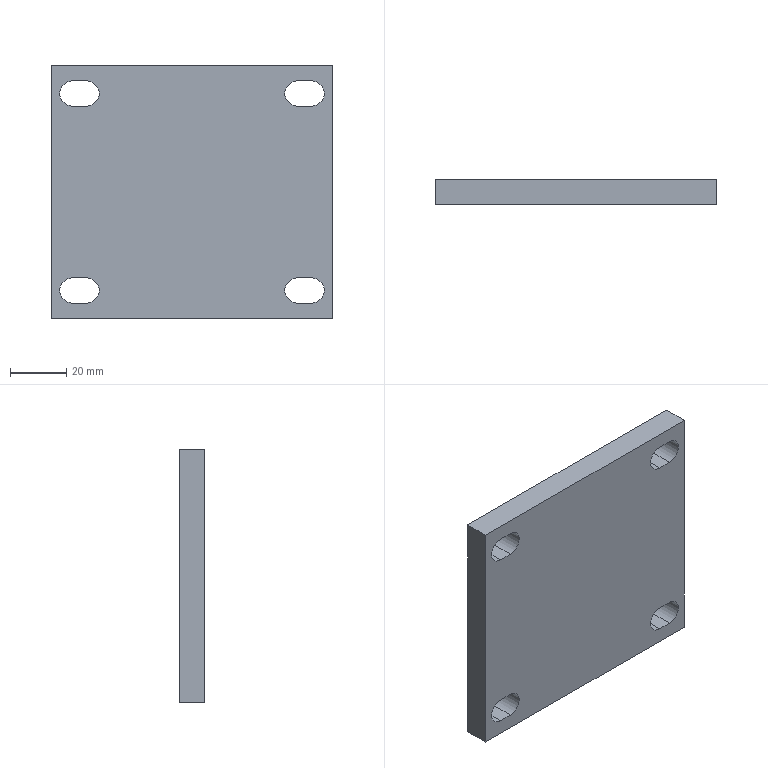Part | STEP file | X77-02211 | 1 solid | 22 faces | box 100 x 9 x 90 mm | volume 77090 mm3 | plane 14 | cylinder 8 | commonest cylinder face diameters 9 x8
STEP:
#1=CARTESIAN_POINT('',(50.,10.,45.));
#2=VERTEX_POINT('',#1);
#3=CARTESIAN_POINT('',(50.,1.,45.));
#4=VERTEX_POINT('',#3);
#5=CARTESIAN_POINT('',(50.,10.,45.));
#6=DIRECTION('',(0.,-1.,0.));
#7=VECTOR('',#6,1000.);
#8=LINE('',#5,#7);
#9=EDGE_CURVE('',#2,#4,#8,.T.);
#10=ORIENTED_EDGE('',*,*,#9,.T.);
#11=CARTESIAN_POINT('',(50.,1.,-45.));
#12=VERTEX_POINT('',#11);
#13=CARTESIAN_POINT('',(50.,1.,45.));
#14=DIRECTION('',(0.,0.,1.));
#15=VECTOR('',#14,1000.);
#16=LINE('',#13,#15);
#17=EDGE_CURVE('',#12,#4,#16,.T.);
#18=ORIENTED_EDGE('',*,*,#17,.F.);
#19=CARTESIAN_POINT('',(50.,10.,-45.));
#20=VERTEX_POINT('',#19);
#21=CARTESIAN_POINT('',(50.,10.,-45.));
#22=DIRECTION('',(0.,-1.,0.));
#23=VECTOR('',#22,1000.);
#24=LINE('',#21,#23);
#25=EDGE_CURVE('',#20,#12,#24,.T.);
#26=ORIENTED_EDGE('',*,*,#25,.F.);
#27=CARTESIAN_POINT('',(50.,10.,45.));
#28=DIRECTION('',(0.,0.,-1.));
#29=VECTOR('',#28,1000.);
#30=LINE('',#27,#29);
#31=EDGE_CURVE('',#2,#20,#30,.T.);
#32=ORIENTED_EDGE('',*,*,#31,.F.);
#33=EDGE_LOOP('',(#10,#18,#26,#32));
#34=FACE_OUTER_BOUND('',#33,.T.);
#35=CARTESIAN_POINT('',(50.,10.,45.));
#36=DIRECTION('',(-1.,0.,0.));
#37=DIRECTION('',(0.,0.,1.));
#38=AXIS2_PLACEMENT_3D('',#35,#36,#37);
#39=PLANE('',#38);
#40=ADVANCED_FACE('',(#34),#39,.F.);
#41=ORIENTED_EDGE('',*,*,#25,.T.);
#42=CARTESIAN_POINT('',(-50.,1.,-45.));
#43=VERTEX_POINT('',#42);
#44=CARTESIAN_POINT('',(-50.,1.,-45.));
#45=DIRECTION('',(1.,0.,0.));
#46=VECTOR('',#45,1000.);
#47=LINE('',#44,#46);
#48=EDGE_CURVE('',#43,#12,#47,.T.);
#49=ORIENTED_EDGE('',*,*,#48,.F.);
#50=CARTESIAN_POINT('',(-50.,10.,-45.));
#51=VERTEX_POINT('',#50);
#52=CARTESIAN_POINT('',(-50.,10.,-45.));
#53=DIRECTION('',(0.,-1.,0.));
#54=VECTOR('',#53,1000.);
#55=LINE('',#52,#54);
#56=EDGE_CURVE('',#51,#43,#55,.T.);
#57=ORIENTED_EDGE('',*,*,#56,.F.);
#58=CARTESIAN_POINT('',(-50.,10.,-45.));
#59=DIRECTION('',(-1.,0.,0.));
#60=VECTOR('',#59,1000.);
#61=LINE('',#58,#60);
#62=EDGE_CURVE('',#20,#51,#61,.T.);
#63=ORIENTED_EDGE('',*,*,#62,.F.);
#64=EDGE_LOOP('',(#41,#49,#57,#63));
#65=FACE_OUTER_BOUND('',#64,.T.);
#66=CARTESIAN_POINT('',(-50.,10.,-45.));
#67=DIRECTION('',(0.,0.,1.));
#68=DIRECTION('',(1.,0.,0.));
#69=AXIS2_PLACEMENT_3D('',#66,#67,#68);
#70=PLANE('',#69);
#71=ADVANCED_FACE('',(#65),#70,.F.);
#72=ORIENTED_EDGE('',*,*,#56,.T.);
#73=CARTESIAN_POINT('',(-50.,1.,45.));
#74=VERTEX_POINT('',#73);
#75=CARTESIAN_POINT('',(-50.,1.,45.));
#76=DIRECTION('',(0.,0.,1.));
#77=VECTOR('',#76,1000.);
#78=LINE('',#75,#77);
#79=EDGE_CURVE('',#43,#74,#78,.T.);
#80=ORIENTED_EDGE('',*,*,#79,.T.);
#81=CARTESIAN_POINT('',(-50.,10.,45.));
#82=VERTEX_POINT('',#81);
#83=CARTESIAN_POINT('',(-50.,10.,45.));
#84=DIRECTION('',(0.,-1.,0.));
#85=VECTOR('',#84,1000.);
#86=LINE('',#83,#85);
#87=EDGE_CURVE('',#82,#74,#86,.T.);
#88=ORIENTED_EDGE('',*,*,#87,.F.);
#89=CARTESIAN_POINT('',(-50.,10.,45.));
#90=DIRECTION('',(0.,0.,1.));
#91=VECTOR('',#90,1000.);
#92=LINE('',#89,#91);
#93=EDGE_CURVE('',#51,#82,#92,.T.);
#94=ORIENTED_EDGE('',*,*,#93,.F.);
#95=EDGE_LOOP('',(#72,#80,#88,#94));
#96=FACE_OUTER_BOUND('',#95,.T.);
#97=CARTESIAN_POINT('',(-50.,10.,45.));
#98=DIRECTION('',(1.,0.,0.));
#99=DIRECTION('',(0.,0.,-1.));
#100=AXIS2_PLACEMENT_3D('',#97,#98,#99);
#101=PLANE('',#100);
#102=ADVANCED_FACE('',(#96),#101,.F.);
#103=ORIENTED_EDGE('',*,*,#87,.T.);
#104=CARTESIAN_POINT('',(-50.,1.,45.));
#105=DIRECTION('',(1.,0.,0.));
#106=VECTOR('',#105,1000.);
#107=LINE('',#104,#106);
#108=EDGE_CURVE('',#74,#4,#107,.T.);
#109=ORIENTED_EDGE('',*,*,#108,.T.);
#110=ORIENTED_EDGE('',*,*,#9,.F.);
#111=CARTESIAN_POINT('',(-50.,10.,45.));
#112=DIRECTION('',(1.,0.,0.));
#113=VECTOR('',#112,1000.);
#114=LINE('',#111,#113);
#115=EDGE_CURVE('',#82,#2,#114,.T.);
#116=ORIENTED_EDGE('',*,*,#115,.F.);
#117=EDGE_LOOP('',(#103,#109,#110,#116));
#118=FACE_OUTER_BOUND('',#117,.T.);
#119=CARTESIAN_POINT('',(-50.,10.,45.));
#120=DIRECTION('',(0.,0.,-1.));
#121=DIRECTION('',(-1.,0.,0.));
#122=AXIS2_PLACEMENT_3D('',#119,#120,#121);
#123=PLANE('',#122);
#124=ADVANCED_FACE('',(#118),#123,.F.);
#125=CARTESIAN_POINT('',(42.5,10.,-39.5));
#126=VERTEX_POINT('',#125);
#127=CARTESIAN_POINT('',(37.5,10.,-39.5));
#128=VERTEX_POINT('',#127);
#129=CARTESIAN_POINT('',(42.5,10.,-39.5));
#130=DIRECTION('',(-1.,0.,0.));
#131=VECTOR('',#130,1000.);
#132=LINE('',#129,#131);
#133=EDGE_CURVE('',#126,#128,#132,.T.);
#134=ORIENTED_EDGE('',*,*,#133,.F.);
#135=CARTESIAN_POINT('',(42.5,10.,-30.5));
#136=VERTEX_POINT('',#135);
#137=CARTESIAN_POINT('',(42.5,10.,-35.));
#138=DIRECTION('',(0.,1.,0.));
#139=DIRECTION('',(0.,0.,1.));
#140=AXIS2_PLACEMENT_3D('',#137,#138,#139);
#141=CIRCLE('',#140,4.5);
#142=EDGE_CURVE('',#136,#126,#141,.T.);
#143=ORIENTED_EDGE('',*,*,#142,.F.);
#144=CARTESIAN_POINT('',(37.5,10.,-30.5));
#145=VERTEX_POINT('',#144);
#146=CARTESIAN_POINT('',(42.5,10.,-30.5));
#147=DIRECTION('',(1.,0.,0.));
#148=VECTOR('',#147,1000.);
#149=LINE('',#146,#148);
#150=EDGE_CURVE('',#145,#136,#149,.T.);
#151=ORIENTED_EDGE('',*,*,#150,.F.);
#152=CARTESIAN_POINT('',(37.5,10.,-35.));
#153=DIRECTION('',(0.,1.,0.));
#154=DIRECTION('',(0.,0.,1.));
#155=AXIS2_PLACEMENT_3D('',#152,#153,#154);
#156=CIRCLE('',#155,4.5);
#157=EDGE_CURVE('',#128,#145,#156,.T.);
#158=ORIENTED_EDGE('',*,*,#157,.F.);
#159=EDGE_LOOP('',(#134,#143,#151,#158));
#160=FACE_BOUND('',#159,.T.);
#161=CARTESIAN_POINT('',(-37.5,10.,-39.5));
#162=VERTEX_POINT('',#161);
#163=CARTESIAN_POINT('',(-42.5,10.,-39.5));
#164=VERTEX_POINT('',#163);
#165=CARTESIAN_POINT('',(-37.5,10.,-39.5));
#166=DIRECTION('',(-1.,0.,0.));
#167=VECTOR('',#166,1000.);
#168=LINE('',#165,#167);
#169=EDGE_CURVE('',#162,#164,#168,.T.);
#170=ORIENTED_EDGE('',*,*,#169,.F.);
#171=CARTESIAN_POINT('',(-37.5,10.,-30.5));
#172=VERTEX_POINT('',#171);
#173=CARTESIAN_POINT('',(-37.5,10.,-35.));
#174=DIRECTION('',(0.,1.,0.));
#175=DIRECTION('',(0.,0.,1.));
#176=AXIS2_PLACEMENT_3D('',#173,#174,#175);
#177=CIRCLE('',#176,4.5);
#178=EDGE_CURVE('',#172,#162,#177,.T.);
#179=ORIENTED_EDGE('',*,*,#178,.F.);
#180=CARTESIAN_POINT('',(-42.5,10.,-30.5));
#181=VERTEX_POINT('',#180);
#182=CARTESIAN_POINT('',(-37.5,10.,-30.5));
#183=DIRECTION('',(1.,0.,0.));
#184=VECTOR('',#183,1000.);
#185=LINE('',#182,#184);
#186=EDGE_CURVE('',#181,#172,#185,.T.);
#187=ORIENTED_EDGE('',*,*,#186,.F.);
#188=CARTESIAN_POINT('',(-42.5,10.,-35.));
#189=DIRECTION('',(0.,1.,0.));
#190=DIRECTION('',(0.,0.,1.));
#191=AXIS2_PLACEMENT_3D('',#188,#189,#190);
#192=CIRCLE('',#191,4.5);
#193=EDGE_CURVE('',#164,#181,#192,.T.);
#194=ORIENTED_EDGE('',*,*,#193,.F.);
#195=EDGE_LOOP('',(#170,#179,#187,#194));
#196=FACE_BOUND('',#195,.T.);
#197=ORIENTED_EDGE('',*,*,#31,.T.);
#198=ORIENTED_EDGE('',*,*,#62,.T.);
#199=ORIENTED_EDGE('',*,*,#93,.T.);
#200=ORIENTED_EDGE('',*,*,#115,.T.);
#201=EDGE_LOOP('',(#197,#198,#199,#200));
#202=FACE_OUTER_BOUND('',#201,.T.);
#203=CARTESIAN_POINT('',(-37.5,10.,39.5));
#204=VERTEX_POINT('',#203);
#205=CARTESIAN_POINT('',(-37.5,10.,30.5));
#206=VERTEX_POINT('',#205);
#207=CARTESIAN_POINT('',(-37.5,10.,35.));
#208=DIRECTION('',(0.,1.,0.));
#209=DIRECTION('',(0.,0.,1.));
#210=AXIS2_PLACEMENT_3D('',#207,#208,#209);
#211=CIRCLE('',#210,4.5);
#212=EDGE_CURVE('',#204,#206,#211,.T.);
#213=ORIENTED_EDGE('',*,*,#212,.F.);
#214=CARTESIAN_POINT('',(-42.5,10.,39.5));
#215=VERTEX_POINT('',#214);
#216=CARTESIAN_POINT('',(-37.5,10.,39.5));
#217=DIRECTION('',(1.,0.,0.));
#218=VECTOR('',#217,1000.);
#219=LINE('',#216,#218);
#220=EDGE_CURVE('',#215,#204,#219,.T.);
#221=ORIENTED_EDGE('',*,*,#220,.F.);
#222=CARTESIAN_POINT('',(-42.5,10.,30.5));
#223=VERTEX_POINT('',#222);
#224=CARTESIAN_POINT('',(-42.5,10.,35.));
#225=DIRECTION('',(0.,1.,0.));
#226=DIRECTION('',(0.,0.,1.));
#227=AXIS2_PLACEMENT_3D('',#224,#225,#226);
#228=CIRCLE('',#227,4.5);
#229=EDGE_CURVE('',#223,#215,#228,.T.);
#230=ORIENTED_EDGE('',*,*,#229,.F.);
#231=CARTESIAN_POINT('',(-37.5,10.,30.5));
#232=DIRECTION('',(-1.,0.,0.));
#233=VECTOR('',#232,1000.);
#234=LINE('',#231,#233);
#235=EDGE_CURVE('',#206,#223,#234,.T.);
#236=ORIENTED_EDGE('',*,*,#235,.F.);
#237=EDGE_LOOP('',(#213,#221,#230,#236));
#238=FACE_BOUND('',#237,.T.);
#239=CARTESIAN_POINT('',(42.5,10.,39.5));
#240=VERTEX_POINT('',#239);
#241=CARTESIAN_POINT('',(42.5,10.,30.5));
#242=VERTEX_POINT('',#241);
#243=CARTESIAN_POINT('',(42.5,10.,35.));
#244=DIRECTION('',(0.,1.,0.));
#245=DIRECTION('',(0.,0.,1.));
#246=AXIS2_PLACEMENT_3D('',#243,#244,#245);
#247=CIRCLE('',#246,4.5);
#248=EDGE_CURVE('',#240,#242,#247,.T.);
#249=ORIENTED_EDGE('',*,*,#248,.F.);
#250=CARTESIAN_POINT('',(37.5,10.,39.5));
#251=VERTEX_POINT('',#250);
#252=CARTESIAN_POINT('',(42.5,10.,39.5));
#253=DIRECTION('',(1.,0.,0.));
#254=VECTOR('',#253,1000.);
#255=LINE('',#252,#254);
#256=EDGE_CURVE('',#251,#240,#255,.T.);
#257=ORIENTED_EDGE('',*,*,#256,.F.);
#258=CARTESIAN_POINT('',(37.5,10.,30.5));
#259=VERTEX_POINT('',#258);
#260=CARTESIAN_POINT('',(37.5,10.,35.));
#261=DIRECTION('',(0.,1.,0.));
#262=DIRECTION('',(0.,0.,1.));
#263=AXIS2_PLACEMENT_3D('',#260,#261,#262);
#264=CIRCLE('',#263,4.5);
#265=EDGE_CURVE('',#259,#251,#264,.T.);
#266=ORIENTED_EDGE('',*,*,#265,.F.);
#267=CARTESIAN_POINT('',(42.5,10.,30.5));
#268=DIRECTION('',(-1.,0.,0.));
#269=VECTOR('',#268,1000.);
#270=LINE('',#267,#269);
#271=EDGE_CURVE('',#242,#259,#270,.T.);
#272=ORIENTED_EDGE('',*,*,#271,.F.);
#273=EDGE_LOOP('',(#249,#257,#266,#272));
#274=FACE_BOUND('',#273,.T.);
#275=CARTESIAN_POINT('',(50.,10.,-45.));
#276=DIRECTION('',(0.,-1.,0.));
#277=DIRECTION('',(0.,0.,-1.));
#278=AXIS2_PLACEMENT_3D('',#275,#276,#277);
#279=PLANE('',#278);
#280=ADVANCED_FACE('',(#160,#196,#202,#238,#274),#279,.F.);
#281=CARTESIAN_POINT('',(-37.5,1.,-39.5));
#282=VERTEX_POINT('',#281);
#283=CARTESIAN_POINT('',(-37.5,0.,-39.5));
#284=DIRECTION('',(0.,1.,0.));
#285=VECTOR('',#284,1000.);
#286=LINE('',#283,#285);
#287=EDGE_CURVE('',#282,#162,#286,.T.);
#288=ORIENTED_EDGE('',*,*,#287,.F.);
#289=CARTESIAN_POINT('',(-37.5,1.,-30.5));
#290=VERTEX_POINT('',#289);
#291=CARTESIAN_POINT('',(-37.5,1.,-35.));
#292=DIRECTION('',(0.,-1.,0.));
#293=DIRECTION('',(0.,0.,1.));
#294=AXIS2_PLACEMENT_3D('',#291,#292,#293);
#295=CIRCLE('',#294,4.5);
#296=EDGE_CURVE('',#282,#290,#295,.T.);
#297=ORIENTED_EDGE('',*,*,#296,.T.);
#298=CARTESIAN_POINT('',(-37.5,0.,-30.5));
#299=DIRECTION('',(0.,1.,0.));
#300=VECTOR('',#299,1000.);
#301=LINE('',#298,#300);
#302=EDGE_CURVE('',#290,#172,#301,.T.);
#303=ORIENTED_EDGE('',*,*,#302,.T.);
#304=ORIENTED_EDGE('',*,*,#178,.T.);
#305=EDGE_LOOP('',(#288,#297,#303,#304));
#306=FACE_OUTER_BOUND('',#305,.T.);
#307=CARTESIAN_POINT('',(-37.5,0.,-35.));
#308=DIRECTION('',(0.,1.,0.));
#309=DIRECTION('',(0.,0.,1.));
#310=AXIS2_PLACEMENT_3D('',#307,#308,#309);
#311=CYLINDRICAL_SURFACE('',#310,4.5);
#312=ADVANCED_FACE('',(#306),#311,.F.);
#313=ORIENTED_EDGE('',*,*,#302,.F.);
#314=CARTESIAN_POINT('',(-42.5,1.,-30.5));
#315=VERTEX_POINT('',#314);
#316=CARTESIAN_POINT('',(-37.5,1.,-30.5));
#317=DIRECTION('',(-1.,0.,0.));
#318=VECTOR('',#317,1000.);
#319=LINE('',#316,#318);
#320=EDGE_CURVE('',#290,#315,#319,.T.);
#321=ORIENTED_EDGE('',*,*,#320,.T.);
#322=CARTESIAN_POINT('',(-42.5,0.,-30.5));
#323=DIRECTION('',(0.,1.,0.));
#324=VECTOR('',#323,1000.);
#325=LINE('',#322,#324);
#326=EDGE_CURVE('',#315,#181,#325,.T.);
#327=ORIENTED_EDGE('',*,*,#326,.T.);
#328=ORIENTED_EDGE('',*,*,#186,.T.);
#329=EDGE_LOOP('',(#313,#321,#327,#328));
#330=FACE_OUTER_BOUND('',#329,.T.);
#331=CARTESIAN_POINT('',(-37.5,0.,-30.5));
#332=DIRECTION('',(0.,0.,1.));
#333=DIRECTION('',(1.,0.,0.));
#334=AXIS2_PLACEMENT_3D('',#331,#332,#333);
#335=PLANE('',#334);
#336=ADVANCED_FACE('',(#330),#335,.F.);
#337=ORIENTED_EDGE('',*,*,#326,.F.);
#338=CARTESIAN_POINT('',(-42.5,1.,-39.5));
#339=VERTEX_POINT('',#338);
#340=CARTESIAN_POINT('',(-42.5,1.,-35.));
#341=DIRECTION('',(0.,-1.,0.));
#342=DIRECTION('',(0.,0.,1.));
#343=AXIS2_PLACEMENT_3D('',#340,#341,#342);
#344=CIRCLE('',#343,4.5);
#345=EDGE_CURVE('',#315,#339,#344,.T.);
#346=ORIENTED_EDGE('',*,*,#345,.T.);
#347=CARTESIAN_POINT('',(-42.5,0.,-39.5));
#348=DIRECTION('',(0.,1.,0.));
#349=VECTOR('',#348,1000.);
#350=LINE('',#347,#349);
#351=EDGE_CURVE('',#339,#164,#350,.T.);
#352=ORIENTED_EDGE('',*,*,#351,.T.);
#353=ORIENTED_EDGE('',*,*,#193,.T.);
#354=EDGE_LOOP('',(#337,#346,#352,#353));
#355=FACE_OUTER_BOUND('',#354,.T.);
#356=CARTESIAN_POINT('',(-42.5,0.,-35.));
#357=DIRECTION('',(0.,1.,0.));
#358=DIRECTION('',(0.,0.,1.));
#359=AXIS2_PLACEMENT_3D('',#356,#357,#358);
#360=CYLINDRICAL_SURFACE('',#359,4.5);
#361=ADVANCED_FACE('',(#355),#360,.F.);
#362=ORIENTED_EDGE('',*,*,#351,.F.);
#363=CARTESIAN_POINT('',(-37.5,1.,-39.5));
#364=DIRECTION('',(1.,0.,0.));
#365=VECTOR('',#364,1000.);
#366=LINE('',#363,#365);
#367=EDGE_CURVE('',#339,#282,#366,.T.);
#368=ORIENTED_EDGE('',*,*,#367,.T.);
#369=ORIENTED_EDGE('',*,*,#287,.T.);
#370=ORIENTED_EDGE('',*,*,#169,.T.);
#371=EDGE_LOOP('',(#362,#368,#369,#370));
#372=FACE_OUTER_BOUND('',#371,.T.);
#373=CARTESIAN_POINT('',(-37.5,0.,-39.5));
#374=DIRECTION('',(0.,0.,-1.));
#375=DIRECTION('',(-1.,0.,0.));
#376=AXIS2_PLACEMENT_3D('',#373,#374,#375);
#377=PLANE('',#376);
#378=ADVANCED_FACE('',(#372),#377,.F.);
#379=CARTESIAN_POINT('',(37.5,1.,-39.5));
#380=VERTEX_POINT('',#379);
#381=CARTESIAN_POINT('',(37.5,0.,-39.5));
#382=DIRECTION('',(0.,1.,0.));
#383=VECTOR('',#382,1000.);
#384=LINE('',#381,#383);
#385=EDGE_CURVE('',#380,#128,#384,.T.);
#386=ORIENTED_EDGE('',*,*,#385,.F.);
#387=CARTESIAN_POINT('',(42.5,1.,-39.5));
#388=VERTEX_POINT('',#387);
#389=CARTESIAN_POINT('',(42.5,1.,-39.5));
#390=DIRECTION('',(1.,0.,0.));
#391=VECTOR('',#390,1000.);
#392=LINE('',#389,#391);
#393=EDGE_CURVE('',#380,#388,#392,.T.);
#394=ORIENTED_EDGE('',*,*,#393,.T.);
#395=CARTESIAN_POINT('',(42.5,0.,-39.5));
#396=DIRECTION('',(0.,1.,0.));
#397=VECTOR('',#396,1000.);
#398=LINE('',#395,#397);
#399=EDGE_CURVE('',#388,#126,#398,.T.);
#400=ORIENTED_EDGE('',*,*,#399,.T.);
#401=ORIENTED_EDGE('',*,*,#133,.T.);
#402=EDGE_LOOP('',(#386,#394,#400,#401));
#403=FACE_OUTER_BOUND('',#402,.T.);
#404=CARTESIAN_POINT('',(42.5,0.,-39.5));
#405=DIRECTION('',(0.,0.,-1.));
#406=DIRECTION('',(-1.,0.,0.));
#407=AXIS2_PLACEMENT_3D('',#404,#405,#406);
#408=PLANE('',#407);
#409=ADVANCED_FACE('',(#403),#408,.F.);
#410=CARTESIAN_POINT('',(37.5,1.,-30.5));
#411=VERTEX_POINT('',#410);
#412=CARTESIAN_POINT('',(37.5,0.,-30.5));
#413=DIRECTION('',(0.,1.,0.));
#414=VECTOR('',#413,1000.);
#415=LINE('',#412,#414);
#416=EDGE_CURVE('',#411,#145,#415,.T.);
#417=ORIENTED_EDGE('',*,*,#416,.F.);
#418=CARTESIAN_POINT('',(37.5,1.,-35.));
#419=DIRECTION('',(0.,-1.,0.));
#420=DIRECTION('',(0.,0.,1.));
#421=AXIS2_PLACEMENT_3D('',#418,#419,#420);
#422=CIRCLE('',#421,4.5);
#423=EDGE_CURVE('',#411,#380,#422,.T.);
#424=ORIENTED_EDGE('',*,*,#423,.T.);
#425=ORIENTED_EDGE('',*,*,#385,.T.);
#426=ORIENTED_EDGE('',*,*,#157,.T.);
#427=EDGE_LOOP('',(#417,#424,#425,#426));
#428=FACE_OUTER_BOUND('',#427,.T.);
#429=CARTESIAN_POINT('',(37.5,0.,-35.));
#430=DIRECTION('',(0.,1.,0.));
#431=DIRECTION('',(0.,0.,1.));
#432=AXIS2_PLACEMENT_3D('',#429,#430,#431);
#433=CYLINDRICAL_SURFACE('',#432,4.5);
#434=ADVANCED_FACE('',(#428),#433,.F.);
#435=CARTESIAN_POINT('',(42.5,1.,-30.5));
#436=VERTEX_POINT('',#435);
#437=CARTESIAN_POINT('',(42.5,0.,-30.5));
#438=DIRECTION('',(0.,1.,0.));
#439=VECTOR('',#438,1000.);
#440=LINE('',#437,#439);
#441=EDGE_CURVE('',#436,#136,#440,.T.);
#442=ORIENTED_EDGE('',*,*,#441,.F.);
#443=CARTESIAN_POINT('',(42.5,1.,-30.5));
#444=DIRECTION('',(-1.,0.,0.));
#445=VECTOR('',#444,1000.);
#446=LINE('',#443,#445);
#447=EDGE_CURVE('',#436,#411,#446,.T.);
#448=ORIENTED_EDGE('',*,*,#447,.T.);
#449=ORIENTED_EDGE('',*,*,#416,.T.);
#450=ORIENTED_EDGE('',*,*,#150,.T.);
#451=EDGE_LOOP('',(#442,#448,#449,#450));
#452=FACE_OUTER_BOUND('',#451,.T.);
#453=CARTESIAN_POINT('',(42.5,0.,-30.5));
#454=DIRECTION('',(0.,0.,1.));
#455=DIRECTION('',(1.,0.,0.));
#456=AXIS2_PLACEMENT_3D('',#453,#454,#455);
#457=PLANE('',#456);
#458=ADVANCED_FACE('',(#452),#457,.F.);
#459=ORIENTED_EDGE('',*,*,#399,.F.);
#460=CARTESIAN_POINT('',(42.5,1.,-35.));
#461=DIRECTION('',(0.,-1.,0.));
#462=DIRECTION('',(0.,0.,1.));
#463=AXIS2_PLACEMENT_3D('',#460,#461,#462);
#464=CIRCLE('',#463,4.5);
#465=EDGE_CURVE('',#388,#436,#464,.T.);
#466=ORIENTED_EDGE('',*,*,#465,.T.);
#467=ORIENTED_EDGE('',*,*,#441,.T.);
#468=ORIENTED_EDGE('',*,*,#142,.T.);
#469=EDGE_LOOP('',(#459,#466,#467,#468));
#470=FACE_OUTER_BOUND('',#469,.T.);
#471=CARTESIAN_POINT('',(42.5,0.,-35.));
#472=DIRECTION('',(0.,1.,0.));
#473=DIRECTION('',(0.,0.,1.));
#474=AXIS2_PLACEMENT_3D('',#471,#472,#473);
#475=CYLINDRICAL_SURFACE('',#474,4.5);
#476=ADVANCED_FACE('',(#470),#475,.F.);
#477=CARTESIAN_POINT('',(-42.5,1.,30.5));
#478=VERTEX_POINT('',#477);
#479=CARTESIAN_POINT('',(-42.5,0.,30.5));
#480=DIRECTION('',(0.,1.,0.));
#481=VECTOR('',#480,1000.);
#482=LINE('',#479,#481);
#483=EDGE_CURVE('',#478,#223,#482,.T.);
#484=ORIENTED_EDGE('',*,*,#483,.F.);
#485=CARTESIAN_POINT('',(-37.5,1.,30.5));
#486=VERTEX_POINT('',#485);
#487=CARTESIAN_POINT('',(-37.5,1.,30.5));
#488=DIRECTION('',(1.,0.,0.));
#489=VECTOR('',#488,1000.);
#490=LINE('',#487,#489);
#491=EDGE_CURVE('',#478,#486,#490,.T.);
#492=ORIENTED_EDGE('',*,*,#491,.T.);
#493=CARTESIAN_POINT('',(-37.5,0.,30.5));
#494=DIRECTION('',(0.,1.,0.));
#495=VECTOR('',#494,1000.);
#496=LINE('',#493,#495);
#497=EDGE_CURVE('',#486,#206,#496,.T.);
#498=ORIENTED_EDGE('',*,*,#497,.T.);
#499=ORIENTED_EDGE('',*,*,#235,.T.);
#500=EDGE_LOOP('',(#484,#492,#498,#499));
#501=FACE_OUTER_BOUND('',#500,.T.);
#502=CARTESIAN_POINT('',(-37.5,0.,30.5));
#503=DIRECTION('',(0.,0.,-1.));
#504=DIRECTION('',(-1.,0.,0.));
#505=AXIS2_PLACEMENT_3D('',#502,#503,#504);
#506=PLANE('',#505);
#507=ADVANCED_FACE('',(#501),#506,.F.);
#508=CARTESIAN_POINT('',(-42.5,1.,39.5));
#509=VERTEX_POINT('',#508);
#510=CARTESIAN_POINT('',(-42.5,0.,39.5));
#511=DIRECTION('',(0.,1.,0.));
#512=VECTOR('',#511,1000.);
#513=LINE('',#510,#512);
#514=EDGE_CURVE('',#509,#215,#513,.T.);
#515=ORIENTED_EDGE('',*,*,#514,.F.);
#516=CARTESIAN_POINT('',(-42.5,1.,35.));
#517=DIRECTION('',(0.,-1.,0.));
#518=DIRECTION('',(0.,0.,1.));
#519=AXIS2_PLACEMENT_3D('',#516,#517,#518);
#520=CIRCLE('',#519,4.5);
#521=EDGE_CURVE('',#509,#478,#520,.T.);
#522=ORIENTED_EDGE('',*,*,#521,.T.);
#523=ORIENTED_EDGE('',*,*,#483,.T.);
#524=ORIENTED_EDGE('',*,*,#229,.T.);
#525=EDGE_LOOP('',(#515,#522,#523,#524));
#526=FACE_OUTER_BOUND('',#525,.T.);
#527=CARTESIAN_POINT('',(-42.5,0.,35.));
#528=DIRECTION('',(0.,1.,0.));
#529=DIRECTION('',(0.,0.,1.));
#530=AXIS2_PLACEMENT_3D('',#527,#528,#529);
#531=CYLINDRICAL_SURFACE('',#530,4.5);
#532=ADVANCED_FACE('',(#526),#531,.F.);
#533=CARTESIAN_POINT('',(-37.5,1.,39.5));
#534=VERTEX_POINT('',#533);
#535=CARTESIAN_POINT('',(-37.5,0.,39.5));
#536=DIRECTION('',(0.,1.,0.));
#537=VECTOR('',#536,1000.);
#538=LINE('',#535,#537);
#539=EDGE_CURVE('',#534,#204,#538,.T.);
#540=ORIENTED_EDGE('',*,*,#539,.F.);
#541=CARTESIAN_POINT('',(-37.5,1.,39.5));
#542=DIRECTION('',(-1.,0.,0.));
#543=VECTOR('',#542,1000.);
#544=LINE('',#541,#543);
#545=EDGE_CURVE('',#534,#509,#544,.T.);
#546=ORIENTED_EDGE('',*,*,#545,.T.);
#547=ORIENTED_EDGE('',*,*,#514,.T.);
#548=ORIENTED_EDGE('',*,*,#220,.T.);
#549=EDGE_LOOP('',(#540,#546,#547,#548));
#550=FACE_OUTER_BOUND('',#549,.T.);
#551=CARTESIAN_POINT('',(-37.5,0.,39.5));
#552=DIRECTION('',(0.,0.,1.));
#553=DIRECTION('',(1.,0.,0.));
#554=AXIS2_PLACEMENT_3D('',#551,#552,#553);
#555=PLANE('',#554);
#556=ADVANCED_FACE('',(#550),#555,.F.);
#557=ORIENTED_EDGE('',*,*,#497,.F.);
#558=CARTESIAN_POINT('',(-37.5,1.,35.));
#559=DIRECTION('',(0.,-1.,0.));
#560=DIRECTION('',(0.,0.,1.));
#561=AXIS2_PLACEMENT_3D('',#558,#559,#560);
#562=CIRCLE('',#561,4.5);
#563=EDGE_CURVE('',#486,#534,#562,.T.);
#564=ORIENTED_EDGE('',*,*,#563,.T.);
#565=ORIENTED_EDGE('',*,*,#539,.T.);
#566=ORIENTED_EDGE('',*,*,#212,.T.);
#567=EDGE_LOOP('',(#557,#564,#565,#566));
#568=FACE_OUTER_BOUND('',#567,.T.);
#569=CARTESIAN_POINT('',(-37.5,0.,35.));
#570=DIRECTION('',(0.,1.,0.));
#571=DIRECTION('',(0.,0.,1.));
#572=AXIS2_PLACEMENT_3D('',#569,#570,#571);
#573=CYLINDRICAL_SURFACE('',#572,4.5);
#574=ADVANCED_FACE('',(#568),#573,.F.);
#575=CARTESIAN_POINT('',(37.5,1.,30.5));
#576=VERTEX_POINT('',#575);
#577=CARTESIAN_POINT('',(37.5,0.,30.5));
#578=DIRECTION('',(0.,1.,0.));
#579=VECTOR('',#578,1000.);
#580=LINE('',#577,#579);
#581=EDGE_CURVE('',#576,#259,#580,.T.);
#582=ORIENTED_EDGE('',*,*,#581,.F.);
#583=CARTESIAN_POINT('',(42.5,1.,30.5));
#584=VERTEX_POINT('',#583);
#585=CARTESIAN_POINT('',(42.5,1.,30.5));
#586=DIRECTION('',(1.,0.,0.));
#587=VECTOR('',#586,1000.);
#588=LINE('',#585,#587);
#589=EDGE_CURVE('',#576,#584,#588,.T.);
#590=ORIENTED_EDGE('',*,*,#589,.T.);
#591=CARTESIAN_POINT('',(42.5,0.,30.5));
#592=DIRECTION('',(0.,1.,0.));
#593=VECTOR('',#592,1000.);
#594=LINE('',#591,#593);
#595=EDGE_CURVE('',#584,#242,#594,.T.);
#596=ORIENTED_EDGE('',*,*,#595,.T.);
#597=ORIENTED_EDGE('',*,*,#271,.T.);
#598=EDGE_LOOP('',(#582,#590,#596,#597));
#599=FACE_OUTER_BOUND('',#598,.T.);
#600=CARTESIAN_POINT('',(42.5,0.,30.5));
#601=DIRECTION('',(0.,0.,-1.));
#602=DIRECTION('',(-1.,0.,0.));
#603=AXIS2_PLACEMENT_3D('',#600,#601,#602);
#604=PLANE('',#603);
#605=ADVANCED_FACE('',(#599),#604,.F.);
#606=CARTESIAN_POINT('',(37.5,1.,39.5));
#607=VERTEX_POINT('',#606);
#608=CARTESIAN_POINT('',(37.5,0.,39.5));
#609=DIRECTION('',(0.,1.,0.));
#610=VECTOR('',#609,1000.);
#611=LINE('',#608,#610);
#612=EDGE_CURVE('',#607,#251,#611,.T.);
#613=ORIENTED_EDGE('',*,*,#612,.F.);
#614=CARTESIAN_POINT('',(37.5,1.,35.));
#615=DIRECTION('',(0.,-1.,0.));
#616=DIRECTION('',(0.,0.,1.));
#617=AXIS2_PLACEMENT_3D('',#614,#615,#616);
#618=CIRCLE('',#617,4.5);
#619=EDGE_CURVE('',#607,#576,#618,.T.);
#620=ORIENTED_EDGE('',*,*,#619,.T.);
#621=ORIENTED_EDGE('',*,*,#581,.T.);
#622=ORIENTED_EDGE('',*,*,#265,.T.);
#623=EDGE_LOOP('',(#613,#620,#621,#622));
#624=FACE_OUTER_BOUND('',#623,.T.);
#625=CARTESIAN_POINT('',(37.5,0.,35.));
#626=DIRECTION('',(0.,1.,0.));
#627=DIRECTION('',(0.,0.,1.));
#628=AXIS2_PLACEMENT_3D('',#625,#626,#627);
#629=CYLINDRICAL_SURFACE('',#628,4.5);
#630=ADVANCED_FACE('',(#624),#629,.F.);
#631=CARTESIAN_POINT('',(42.5,1.,39.5));
#632=VERTEX_POINT('',#631);
#633=CARTESIAN_POINT('',(42.5,0.,39.5));
#634=DIRECTION('',(0.,1.,0.));
#635=VECTOR('',#634,1000.);
#636=LINE('',#633,#635);
#637=EDGE_CURVE('',#632,#240,#636,.T.);
#638=ORIENTED_EDGE('',*,*,#637,.F.);
#639=CARTESIAN_POINT('',(42.5,1.,39.5));
#640=DIRECTION('',(-1.,0.,0.));
#641=VECTOR('',#640,1000.);
#642=LINE('',#639,#641);
#643=EDGE_CURVE('',#632,#607,#642,.T.);
#644=ORIENTED_EDGE('',*,*,#643,.T.);
#645=ORIENTED_EDGE('',*,*,#612,.T.);
#646=ORIENTED_EDGE('',*,*,#256,.T.);
#647=EDGE_LOOP('',(#638,#644,#645,#646));
#648=FACE_OUTER_BOUND('',#647,.T.);
#649=CARTESIAN_POINT('',(42.5,0.,39.5));
#650=DIRECTION('',(0.,0.,1.));
#651=DIRECTION('',(1.,0.,0.));
#652=AXIS2_PLACEMENT_3D('',#649,#650,#651);
#653=PLANE('',#652);
#654=ADVANCED_FACE('',(#648),#653,.F.);
#655=ORIENTED_EDGE('',*,*,#595,.F.);
#656=CARTESIAN_POINT('',(42.5,1.,35.));
#657=DIRECTION('',(0.,-1.,0.));
#658=DIRECTION('',(0.,0.,1.));
#659=AXIS2_PLACEMENT_3D('',#656,#657,#658);
#660=CIRCLE('',#659,4.5);
#661=EDGE_CURVE('',#584,#632,#660,.T.);
#662=ORIENTED_EDGE('',*,*,#661,.T.);
#663=ORIENTED_EDGE('',*,*,#637,.T.);
#664=ORIENTED_EDGE('',*,*,#248,.T.);
#665=EDGE_LOOP('',(#655,#662,#663,#664));
#666=FACE_OUTER_BOUND('',#665,.T.);
#667=CARTESIAN_POINT('',(42.5,0.,35.));
#668=DIRECTION('',(0.,1.,0.));
#669=DIRECTION('',(0.,0.,1.));
#670=AXIS2_PLACEMENT_3D('',#667,#668,#669);
#671=CYLINDRICAL_SURFACE('',#670,4.5);
#672=ADVANCED_FACE('',(#666),#671,.F.);
#673=ORIENTED_EDGE('',*,*,#17,.T.);
#674=ORIENTED_EDGE('',*,*,#108,.F.);
#675=ORIENTED_EDGE('',*,*,#79,.F.);
#676=ORIENTED_EDGE('',*,*,#48,.T.);
#677=EDGE_LOOP('',(#673,#674,#675,#676));
#678=FACE_OUTER_BOUND('',#677,.T.);
#679=ORIENTED_EDGE('',*,*,#619,.F.);
#680=ORIENTED_EDGE('',*,*,#643,.F.);
#681=ORIENTED_EDGE('',*,*,#661,.F.);
#682=ORIENTED_EDGE('',*,*,#589,.F.);
#683=EDGE_LOOP('',(#679,#680,#681,#682));
#684=FACE_BOUND('',#683,.T.);
#685=ORIENTED_EDGE('',*,*,#521,.F.);
#686=ORIENTED_EDGE('',*,*,#545,.F.);
#687=ORIENTED_EDGE('',*,*,#563,.F.);
#688=ORIENTED_EDGE('',*,*,#491,.F.);
#689=EDGE_LOOP('',(#685,#686,#687,#688));
#690=FACE_BOUND('',#689,.T.);
#691=ORIENTED_EDGE('',*,*,#393,.F.);
#692=ORIENTED_EDGE('',*,*,#423,.F.);
#693=ORIENTED_EDGE('',*,*,#447,.F.);
#694=ORIENTED_EDGE('',*,*,#465,.F.);
#695=EDGE_LOOP('',(#691,#692,#693,#694));
#696=FACE_BOUND('',#695,.T.);
#697=ORIENTED_EDGE('',*,*,#367,.F.);
#698=ORIENTED_EDGE('',*,*,#345,.F.);
#699=ORIENTED_EDGE('',*,*,#320,.F.);
#700=ORIENTED_EDGE('',*,*,#296,.F.);
#701=EDGE_LOOP('',(#697,#698,#699,#700));
#702=FACE_BOUND('',#701,.T.);
#703=CARTESIAN_POINT('',(-50.,1.,45.));
#704=DIRECTION('',(0.,1.,0.));
#705=DIRECTION('',(0.,0.,1.));
#706=AXIS2_PLACEMENT_3D('',#703,#704,#705);
#707=PLANE('',#706);
#708=ADVANCED_FACE('',(#678,#684,#690,#696,#702),#707,.F.);
#709=CLOSED_SHELL('',(#40,#71,#102,#124,#280,#312,#336,#361,#378,#409,#434,#458,#476,#507,#532,#556,#574,#605,#630,#654,#672,#708));
#710=MANIFOLD_SOLID_BREP('',#709);
#711=CARTESIAN_POINT('',(0.,0.,0.));
#712=DIRECTION('',(0.,0.,1.));
#713=DIRECTION('',(1.,0.,0.));
#714=AXIS2_PLACEMENT_3D('',#711,#712,#713);
#715=(LENGTH_UNIT()NAMED_UNIT(*)SI_UNIT(.MILLI.,.METRE.));
#716=UNCERTAINTY_MEASURE_WITH_UNIT(LENGTH_MEASURE(0.00001),#715,'','');
#717=(NAMED_UNIT(*)PLANE_ANGLE_UNIT()SI_UNIT($,.RADIAN.));
#718=(NAMED_UNIT(*)SI_UNIT($,.STERADIAN.)SOLID_ANGLE_UNIT());
#719=(GEOMETRIC_REPRESENTATION_CONTEXT(3)GLOBAL_UNCERTAINTY_ASSIGNED_CONTEXT((#716))GLOBAL_UNIT_ASSIGNED_CONTEXT((#715,#717,#718))REPRESENTATION_CONTEXT('',''));
#720=ADVANCED_BREP_SHAPE_REPRESENTATION('',(#710,#714),#719);